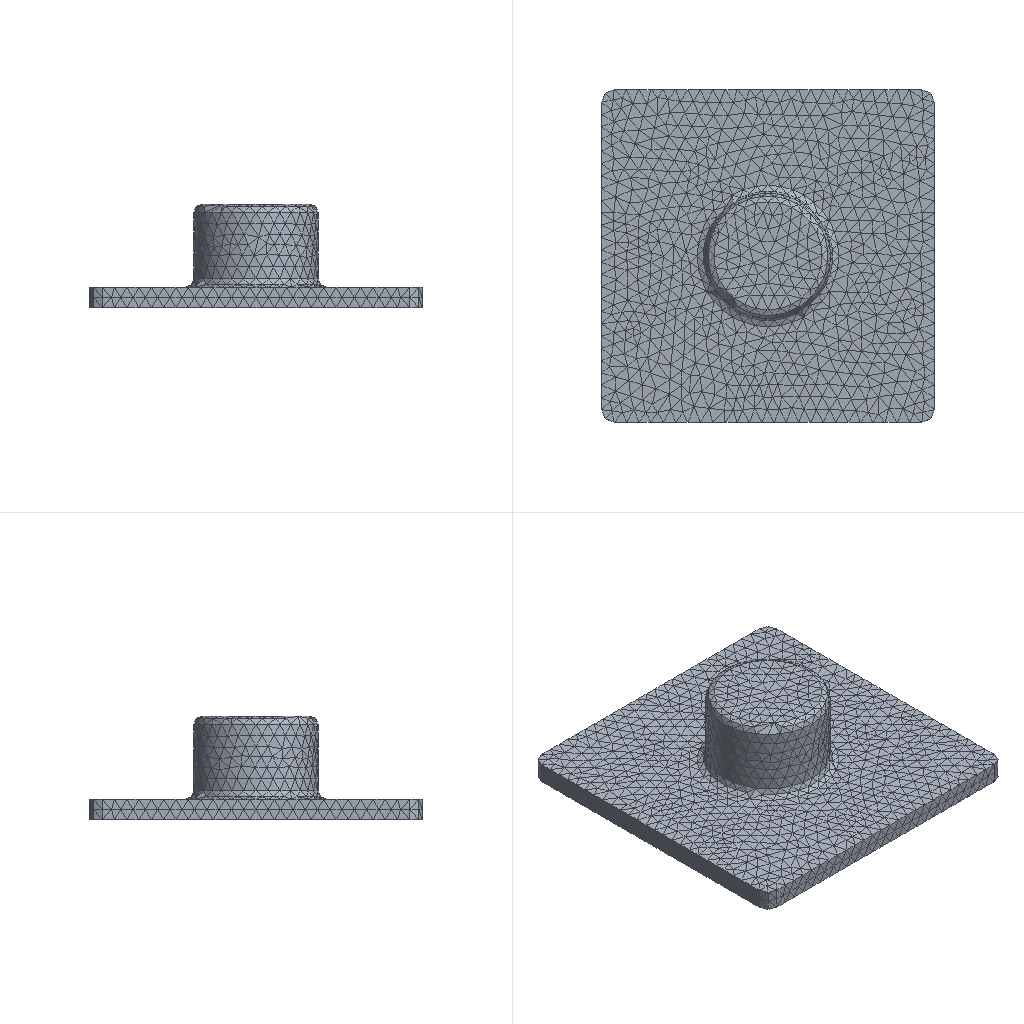Simulation study | ansys workbench
Ansys APDL input file, long lists of numbers shortened:
/batch
/config,noeldb,1     ! force off writing results to database
*get,_wallstrt,active,,time,wall
! ANSYS input file written by Workbench version 2024 R2
! File used for geometry attach:
/title,wbnew--____ (B5)
! ****** Begin Custom Load Command Snippet ******
/COM, ACT Extensions:
/COM,     LSDYNA, 2024.2
/COM,/COM,     ANSYSMotion, 2024.2
/COM,
! ****** End   Custom Load Command Snippet ******
*DIM,_wb_ProjectScratch_dir,string,248
_wb_ProjectScratch_dir(1) = ''
*DIM,_wb_SolverFiles_dir,string,248
_wb_SolverFiles_dir(1) = ''
*DIM,_wb_userfiles_dir,string,248
_wb_userfiles_dir(1) = ''
/com,--- Data in consistent NMM units. See Solving Units in the help system for more information.
/units,MPA
/nopr
/wb,file,start              !  signify a WB generated input file
/prep7
! Turn off shape checking because checks already performed inside WB mesher.
! See help system for more information.
SHPP,OFF,,NOWARN
/nolist
etcon,set             ! allow ANSYS to choose best KEYOP's for 180x elements, resets any applicable keyopt to MAPDL defaults
/com,*********** Nodes for the whole assembly ***********
nblock,3,,26937
(1i9,3e20.9e3)
        1     2.555492712E+03     4.188182850E+03     2.300000000E+01
! (24488 more lines like these left out)
-1
/wb,elem,start            !  set before creation of elements
/com,*********** Elements for Body 1 'Part 1' ***********
et,1,187
eblock,19,solid,,15247
(19i9)
        1        1        1        1        0        0        0        0       10        0        1     2372     3619     2402     3612    19388    19523    19383    19387
! (30493 more lines like these left out)
-1
/wb,elem,end               !  done creating elements
/com,*********** Send User Defined Coordinate System(s) ***********
csys,0
toffst,273.15,      ! Temperature offset from absolute zero
/com,*********** Set Reference Temperature ***********
tref,22.
/wb,mat,start              !  starting to send materials
/com,*********** Send Materials ***********
Temperature = 'TEMP' ! Temperature
MP,DENS,1,7.85e-09,	! tonne mm^-3
MP,ALPX,1,1.2e-05,	! C^-1
MP,C,1,434000000,	! mm^2 s^-2 C^-1
MP,KXX,1,60.5,	! tonne mm s^-3 C^-1
MP,RSVX,1,0.00017,	! ohm mm
MP,EX,1,200000,	! tonne s^-2 mm^-1
MP,NUXY,1,0.3,
MP,MURX,1,10000,
/wb,mat,end                !  done sending materials
!************************* Model Summary ********************
!Part 1,	结构钢,	matid,	1
!************************* End Model Summary ********************
! get the diagonal of the bounding box. Needed later for other things
*get,_xmin,node,,mnloc,x
*get,_ymin,node,,mnloc,y
*get,_zmin,node,,mnloc,z
*get,_xmax,node,,mxloc,x
*get,_ymax,node,,mxloc,y
*get,_zmax,node,,mxloc,z
_ASMDIAG=(_xmax-_xmin)*(_xmax-_xmin)+(_ymax-_ymin)*(_ymax-_ymin)+(_zmax-_zmin)*(_zmax-_zmin)
_ASMDIAG=SQRT(_ASMDIAG)
/wb,contact,start          !  starting to send contact
/wb,contact,end            !  done creating contacts
/golist
/wb,load,start             !  starting to send loads
/com,*********** Fixed Supports ***********
CMBLOCK,_FIXEDSU,NODE,     3125
(8i10)
       237       238       239       242       243       244       245       246
! (390 more lines like these left out)
cmsel,s,_FIXEDSU
d,all,all
nsel,all
/gst,on,on
fini
*get,_numnode,node,0,count
*get,_numelem,elem,0,count
*get, _MAXELEMNUM, elem, 0, NUM, MAX
*get, _MAXNODENUM, node, 0, NUM, MAX
*get, _MAXELEMTYPE, etyp, 0, NUM, MAX
*get, _MAXREALCONST, rcon, 0, NUM, MAX
/go
/wb,load,end               !  done creating loads
/com,--- Number of total nodes = %_numnode%
/com,--- Number of contact elements = 0
/com,--- Number of spring elements = 0
/com,--- Number of bearing elements = 0
/com,--- Number of solid elements = 15247
/com,--- Number of condensed parts = 0
/com,--- Number of total elements = %_numelem%
*get,_wallbsol,active,,time,wall
/com,****************************************************************************
/com,*************************    SOLUTION       ********************************
/com,****************************************************************************
/solu
antype,0                   ! static analysis
_thickRatio=  1     ! Ratio of thick parts in the model
eqsl,pcg,1e-8,,,,,,1
cntr,print,1               ! print out contact info and also make no initial contact an error
cncheck,dmp		!	Enable program controlled contact splitting for distributed memory parallel run
dmpoption,emat,no             ! Don't combine emat file for DANSYS
dmpoption,esav,no             ! Don't combine esav file for DANSYS
nldiag,cont,iter           ! print out contact info each equilibrium iteration
rescontrol,,none                 ! Do not keep any restart files
/com,****************************************************
/com,******************* SOLVE FOR LS 1 OF 1 ****************
/nopr
/com,*********** Create Imported Load "________" ***********
/nopr
bfblock,2,temp,24489,24489,0
(i9,e20.9e3)
        1     8.000000000e+01
! (24488 more lines like these left out)
bf,end,loc,-1,
/gopr
/gopr
nsub,1,1,1
time,1.
outres,erase
outres,all,none
outres,nsol,all,
outres,rsol,all
outres,eangl,all
outres,etmp,all
outres,veng,all
outres,strs,all,
outres,epel,all,
outres,eppl,all,
outres,epth,all,
outres,cont,all,
! *********** WB SOLVE COMMAND ***********
! check interactive state
*get,ANSINTER_,active,,int
*if,ANSINTER_,ne,0,then
/eof
*endif
solve
/com *************** Write FE CONNECTORS *********
CEWRITE,file,ce,,INTE
/com,****************************************************
/com,*************** FINISHED SOLVE FOR LS 1 *************
*get,_wallasol,active,,time,wall
/nopr
*get,_numnode,node,0,count
*get,_numelem,elem,0,count
*get, _MAXELEMNUM, elem, 0, NUM, MAX
*get, _MAXNODENUM, node, 0, NUM, MAX,,,INTERNAL
*get, _MAXELEMTYPE, etyp, 0, NUM, MAX
*get, _MAXREALCONST, rcon, 0, NUM, MAX
*get,_NSOLTHREADS,active,0,ntfs
*get,_NSOLPROCESSES,active,0,npfs
/gopr
*get,_PCGITER,active,,solu,cgiter
/post1
xmlo,ENCODING,ISO-8859-1
xmlo,parm
/xml,parm,xml
fini
/gopr
*get,_walldone,active,,time,wall
_preptime=(_wallbsol-_wallstrt)*3600
_solvtime=(_wallasol-_wallbsol)*3600
_posttime=(_walldone-_wallasol)*3600
_totaltim=(_walldone-_wallstrt)*3600
*get,_dlbratio,active,0,solu,dlbr
*get,_combtime,active,0,solu,comb
*get,_ssmode,active,0,solu,ssmm
*get,_ndofs,active,0,solu,ndof
*get,_sol_end_time,active,0,set,time
*if,_sol_end_time,eq,1.,then
/fclean				!clean distributed files
*endif
/com,--- Total number of nodes = %_numnode%
/com,--- Total number of elements = %_numelem%
/com,--- Element load balance ratio = %_dlbratio%
/com,--- Time to combine distributed files = %_combtime%
/com,--- Sparse memory mode = %_ssmode%
/com,--- Number of DOF = %_ndofs%
/wb,file,end               ! done with WB generated input